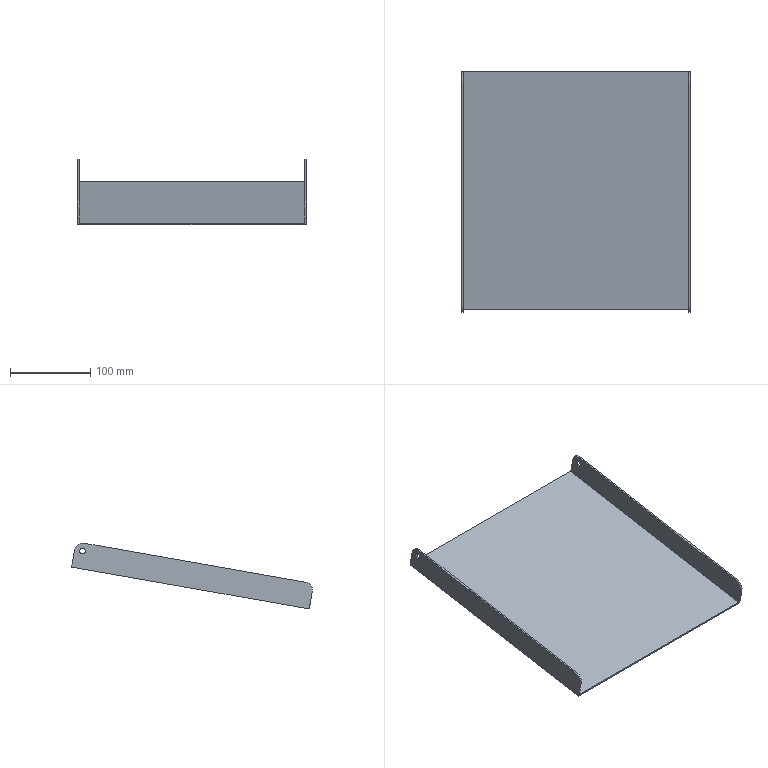Part | NX | features HB 2 | 1 solid | 16 faces | box 285 x 300.028 x 82.132 mm | volume 207104 mm3 | plane 10 | cylinder 6 | commonest cylinder face diameters 20 x4 7 x2
STEP:
#1=CARTESIAN_POINT('',(564.,-684.707,-373.956));
#2=VERTEX_POINT('',#1);
#3=CARTESIAN_POINT('',(564.,-685.612,-377.336));
#4=DIRECTION('',(1.,0.,0.));
#5=DIRECTION('',(0.,0.2588,0.9659));
#6=AXIS2_PLACEMENT_3D('',#3,#4,#5);
#7=CIRCLE('',#6,3.5);
#8=EDGE_CURVE('',#2,#2,#7,.T.);
#9=ORIENTED_EDGE('',*,*,#8,.F.);
#10=EDGE_LOOP('',(#9));
#11=FACE_BOUND('',#10,.T.);
#12=CARTESIAN_POINT('',(566.,-684.707,-373.956));
#13=VERTEX_POINT('',#12);
#14=CARTESIAN_POINT('',(566.,-685.612,-377.336));
#15=DIRECTION('',(-1.,0.,0.));
#16=DIRECTION('',(0.,0.2588,0.9659));
#17=AXIS2_PLACEMENT_3D('',#14,#15,#16);
#18=CIRCLE('',#17,3.5);
#19=EDGE_CURVE('',#13,#13,#18,.T.);
#20=ORIENTED_EDGE('',*,*,#19,.F.);
#21=EDGE_LOOP('',(#20));
#22=FACE_BOUND('',#21,.T.);
#23=CARTESIAN_POINT('',(1166.,-685.612,-377.336));
#24=DIRECTION('',(-1.,0.,0.));
#25=DIRECTION('',(0.,-0.2588,-0.9659));
#26=AXIS2_PLACEMENT_3D('',#23,#24,#25);
#27=CYLINDRICAL_SURFACE('',#26,3.5);
#28=ADVANCED_FACE('',(#11,#22),#27,.F.);
#29=CARTESIAN_POINT('',(564.,-687.349,-367.488));
#30=VERTEX_POINT('',#29);
#31=CARTESIAN_POINT('',(564.,-963.709,-416.218));
#32=VERTEX_POINT('',#31);
#33=CARTESIAN_POINT('',(564.,-562.892,-345.543));
#34=DIRECTION('',(0.,-0.9848,-0.1736));
#35=VECTOR('',#34,1000.);
#36=LINE('',#33,#35);
#37=EDGE_CURVE('',#30,#32,#36,.T.);
#38=ORIENTED_EDGE('',*,*,#37,.T.);
#39=CARTESIAN_POINT('',(566.,-963.709,-416.218));
#40=VERTEX_POINT('',#39);
#41=CARTESIAN_POINT('',(560.,-963.709,-416.218));
#42=DIRECTION('',(1.,0.,0.));
#43=VECTOR('',#42,1000.);
#44=LINE('',#41,#43);
#45=EDGE_CURVE('',#32,#40,#44,.T.);
#46=ORIENTED_EDGE('',*,*,#45,.T.);
#47=CARTESIAN_POINT('',(566.,-687.349,-367.488));
#48=VERTEX_POINT('',#47);
#49=CARTESIAN_POINT('',(566.,-562.892,-345.543));
#50=DIRECTION('',(0.,-0.9848,-0.1736));
#51=VECTOR('',#50,1000.);
#52=LINE('',#49,#51);
#53=EDGE_CURVE('',#48,#40,#52,.T.);
#54=ORIENTED_EDGE('',*,*,#53,.F.);
#55=CARTESIAN_POINT('',(560.,-687.349,-367.488));
#56=DIRECTION('',(1.,0.,0.));
#57=VECTOR('',#56,1000.);
#58=LINE('',#55,#57);
#59=EDGE_CURVE('',#30,#48,#58,.T.);
#60=ORIENTED_EDGE('',*,*,#59,.F.);
#61=EDGE_LOOP('',(#38,#46,#54,#60));
#62=FACE_BOUND('',#61,.T.);
#63=CARTESIAN_POINT('',(560.,-562.892,-345.543));
#64=DIRECTION('',(0.,0.1736,-0.9848));
#65=DIRECTION('',(0.,-0.9848,-0.1736));
#66=AXIS2_PLACEMENT_3D('',#63,#64,#65);
#67=PLANE('',#66);
#68=ADVANCED_FACE('',(#62),#67,.F.);
#69=CARTESIAN_POINT('',(564.,-971.82,-427.803));
#70=VERTEX_POINT('',#69);
#71=CARTESIAN_POINT('',(564.,-961.972,-426.066));
#72=DIRECTION('',(-1.,0.,0.));
#73=DIRECTION('',(0.,0.2588,0.9659));
#74=AXIS2_PLACEMENT_3D('',#71,#72,#73);
#75=CIRCLE('',#74,10.);
#76=EDGE_CURVE('',#70,#32,#75,.T.);
#77=ORIENTED_EDGE('',*,*,#76,.F.);
#78=CARTESIAN_POINT('',(566.,-971.82,-427.803));
#79=VERTEX_POINT('',#78);
#80=CARTESIAN_POINT('',(520.,-971.82,-427.803));
#81=DIRECTION('',(-1.,0.,0.));
#82=VECTOR('',#81,1000.);
#83=LINE('',#80,#82);
#84=EDGE_CURVE('',#79,#70,#83,.T.);
#85=ORIENTED_EDGE('',*,*,#84,.F.);
#86=CARTESIAN_POINT('',(566.,-961.972,-426.066));
#87=DIRECTION('',(1.,0.,0.));
#88=DIRECTION('',(0.,0.2588,0.9659));
#89=AXIS2_PLACEMENT_3D('',#86,#87,#88);
#90=CIRCLE('',#89,10.);
#91=EDGE_CURVE('',#40,#79,#90,.T.);
#92=ORIENTED_EDGE('',*,*,#91,.F.);
#93=ORIENTED_EDGE('',*,*,#45,.F.);
#94=EDGE_LOOP('',(#77,#85,#92,#93));
#95=FACE_BOUND('',#94,.T.);
#96=CARTESIAN_POINT('',(560.,-961.972,-426.066));
#97=DIRECTION('',(1.,0.,0.));
#98=DIRECTION('',(0.,0.2588,0.9659));
#99=AXIS2_PLACEMENT_3D('',#96,#97,#98);
#100=CYLINDRICAL_SURFACE('',#99,10.);
#101=ADVANCED_FACE('',(#95),#100,.T.);
#102=ORIENTED_EDGE('',*,*,#53,.T.);
#103=ORIENTED_EDGE('',*,*,#91,.T.);
#104=CARTESIAN_POINT('',(566.,-968.,-449.468));
#105=VERTEX_POINT('',#104);
#106=CARTESIAN_POINT('',(566.,-968.347,-447.499));
#107=DIRECTION('',(0.,0.1736,-0.9848));
#108=VECTOR('',#107,1000.);
#109=LINE('',#106,#108);
#110=EDGE_CURVE('',#79,#105,#109,.T.);
#111=ORIENTED_EDGE('',*,*,#110,.T.);
#112=CARTESIAN_POINT('',(566.,-671.944,-397.266));
#113=VERTEX_POINT('',#112);
#114=CARTESIAN_POINT('',(566.,-557.335,-377.057));
#115=DIRECTION('',(0.,0.9848,0.1736));
#116=VECTOR('',#115,1000.);
#117=LINE('',#114,#116);
#118=EDGE_CURVE('',#105,#113,#117,.T.);
#119=ORIENTED_EDGE('',*,*,#118,.T.);
#120=CARTESIAN_POINT('',(566.,-675.764,-375.6));
#121=VERTEX_POINT('',#120);
#122=CARTESIAN_POINT('',(566.,-672.291,-395.296));
#123=DIRECTION('',(0.,0.1736,-0.9848));
#124=VECTOR('',#123,1000.);
#125=LINE('',#122,#124);
#126=EDGE_CURVE('',#121,#113,#125,.T.);
#127=ORIENTED_EDGE('',*,*,#126,.F.);
#128=CARTESIAN_POINT('',(566.,-685.612,-377.336));
#129=DIRECTION('',(-1.,0.,0.));
#130=DIRECTION('',(0.,-0.5736,0.8192));
#131=AXIS2_PLACEMENT_3D('',#128,#129,#130);
#132=CIRCLE('',#131,10.);
#133=EDGE_CURVE('',#48,#121,#132,.T.);
#134=ORIENTED_EDGE('',*,*,#133,.F.);
#135=EDGE_LOOP('',(#102,#103,#111,#119,#127,#134));
#136=FACE_BOUND('',#135,.T.);
#137=ORIENTED_EDGE('',*,*,#19,.T.);
#138=EDGE_LOOP('',(#137));
#139=FACE_BOUND('',#138,.T.);
#140=CARTESIAN_POINT('',(566.,-557.683,-375.087));
#141=DIRECTION('',(-1.,0.,0.));
#142=DIRECTION('',(0.,-0.2588,-0.9659));
#143=AXIS2_PLACEMENT_3D('',#140,#141,#142);
#144=PLANE('',#143);
#145=ADVANCED_FACE('',(#136,#139),#144,.F.);
#146=CARTESIAN_POINT('',(564.,-675.764,-375.6));
#147=VERTEX_POINT('',#146);
#148=CARTESIAN_POINT('',(564.,-685.612,-377.336));
#149=DIRECTION('',(1.,0.,0.));
#150=DIRECTION('',(0.,-0.5736,0.8192));
#151=AXIS2_PLACEMENT_3D('',#148,#149,#150);
#152=CIRCLE('',#151,10.);
#153=EDGE_CURVE('',#147,#30,#152,.T.);
#154=ORIENTED_EDGE('',*,*,#153,.T.);
#155=ORIENTED_EDGE('',*,*,#59,.T.);
#156=ORIENTED_EDGE('',*,*,#133,.T.);
#157=CARTESIAN_POINT('',(560.,-675.764,-375.6));
#158=DIRECTION('',(-1.,0.,0.));
#159=VECTOR('',#158,1000.);
#160=LINE('',#157,#159);
#161=EDGE_CURVE('',#121,#147,#160,.T.);
#162=ORIENTED_EDGE('',*,*,#161,.T.);
#163=EDGE_LOOP('',(#154,#155,#156,#162));
#164=FACE_BOUND('',#163,.T.);
#165=CARTESIAN_POINT('',(560.,-685.612,-377.336));
#166=DIRECTION('',(1.,0.,0.));
#167=DIRECTION('',(0.,-0.5736,0.8192));
#168=AXIS2_PLACEMENT_3D('',#165,#166,#167);
#169=CYLINDRICAL_SURFACE('',#168,10.);
#170=ADVANCED_FACE('',(#164),#169,.T.);
#171=ORIENTED_EDGE('',*,*,#76,.T.);
#172=ORIENTED_EDGE('',*,*,#37,.F.);
#173=ORIENTED_EDGE('',*,*,#153,.F.);
#174=CARTESIAN_POINT('',(564.,-672.291,-395.296));
#175=VERTEX_POINT('',#174);
#176=CARTESIAN_POINT('',(564.,-672.291,-395.296));
#177=DIRECTION('',(0.,0.1736,-0.9848));
#178=VECTOR('',#177,1000.);
#179=LINE('',#176,#178);
#180=EDGE_CURVE('',#147,#175,#179,.T.);
#181=ORIENTED_EDGE('',*,*,#180,.T.);
#182=CARTESIAN_POINT('',(564.,-968.347,-447.499));
#183=VERTEX_POINT('',#182);
#184=CARTESIAN_POINT('',(564.,-557.683,-375.087));
#185=DIRECTION('',(0.,-0.9848,-0.1736));
#186=VECTOR('',#185,1000.);
#187=LINE('',#184,#186);
#188=EDGE_CURVE('',#175,#183,#187,.T.);
#189=ORIENTED_EDGE('',*,*,#188,.T.);
#190=CARTESIAN_POINT('',(564.,-968.347,-447.499));
#191=DIRECTION('',(0.,0.1736,-0.9848));
#192=VECTOR('',#191,1000.);
#193=LINE('',#190,#192);
#194=EDGE_CURVE('',#70,#183,#193,.T.);
#195=ORIENTED_EDGE('',*,*,#194,.F.);
#196=EDGE_LOOP('',(#171,#172,#173,#181,#189,#195));
#197=FACE_BOUND('',#196,.T.);
#198=ORIENTED_EDGE('',*,*,#8,.T.);
#199=EDGE_LOOP('',(#198));
#200=FACE_BOUND('',#199,.T.);
#201=CARTESIAN_POINT('',(564.,-557.683,-375.087));
#202=DIRECTION('',(-1.,0.,0.));
#203=DIRECTION('',(0.,0.2588,0.9659));
#204=AXIS2_PLACEMENT_3D('',#201,#202,#203);
#205=PLANE('',#204);
#206=ADVANCED_FACE('',(#197,#200),#205,.T.);
#207=CARTESIAN_POINT('',(283.,-672.291,-395.296));
#208=VERTEX_POINT('',#207);
#209=CARTESIAN_POINT('',(520.,-672.291,-395.296));
#210=DIRECTION('',(1.,0.,0.));
#211=VECTOR('',#210,1000.);
#212=LINE('',#209,#211);
#213=EDGE_CURVE('',#208,#175,#212,.T.);
#214=ORIENTED_EDGE('',*,*,#213,.T.);
#215=ORIENTED_EDGE('',*,*,#180,.F.);
#216=ORIENTED_EDGE('',*,*,#161,.F.);
#217=ORIENTED_EDGE('',*,*,#126,.T.);
#218=CARTESIAN_POINT('',(281.,-671.944,-397.266));
#219=VERTEX_POINT('',#218);
#220=CARTESIAN_POINT('',(520.,-671.944,-397.266));
#221=DIRECTION('',(1.,0.,0.));
#222=VECTOR('',#221,1000.);
#223=LINE('',#220,#222);
#224=EDGE_CURVE('',#219,#113,#223,.T.);
#225=ORIENTED_EDGE('',*,*,#224,.F.);
#226=CARTESIAN_POINT('',(281.,-675.764,-375.6));
#227=VERTEX_POINT('',#226);
#228=CARTESIAN_POINT('',(281.,-672.291,-395.296));
#229=DIRECTION('',(0.,0.1736,-0.9848));
#230=VECTOR('',#229,1000.);
#231=LINE('',#228,#230);
#232=EDGE_CURVE('',#227,#219,#231,.T.);
#233=ORIENTED_EDGE('',*,*,#232,.F.);
#234=CARTESIAN_POINT('',(283.,-675.764,-375.6));
#235=VERTEX_POINT('',#234);
#236=CARTESIAN_POINT('',(586.,-675.764,-375.6));
#237=DIRECTION('',(-1.,0.,0.));
#238=VECTOR('',#237,1000.);
#239=LINE('',#236,#238);
#240=EDGE_CURVE('',#235,#227,#239,.T.);
#241=ORIENTED_EDGE('',*,*,#240,.F.);
#242=CARTESIAN_POINT('',(283.,-672.291,-395.296));
#243=DIRECTION('',(0.,0.1736,-0.9848));
#244=VECTOR('',#243,1000.);
#245=LINE('',#242,#244);
#246=EDGE_CURVE('',#235,#208,#245,.T.);
#247=ORIENTED_EDGE('',*,*,#246,.T.);
#248=EDGE_LOOP('',(#214,#215,#216,#217,#225,#233,#241,#247));
#249=FACE_BOUND('',#248,.T.);
#250=CARTESIAN_POINT('',(520.,-672.291,-395.296));
#251=DIRECTION('',(0.,-0.9848,-0.1736));
#252=DIRECTION('',(0.,0.1736,-0.9848));
#253=AXIS2_PLACEMENT_3D('',#250,#251,#252);
#254=PLANE('',#253);
#255=ADVANCED_FACE('',(#249),#254,.F.);
#256=ORIENTED_EDGE('',*,*,#194,.T.);
#257=CARTESIAN_POINT('',(283.,-968.347,-447.499));
#258=VERTEX_POINT('',#257);
#259=CARTESIAN_POINT('',(520.,-968.347,-447.499));
#260=DIRECTION('',(1.,0.,0.));
#261=VECTOR('',#260,1000.);
#262=LINE('',#259,#261);
#263=EDGE_CURVE('',#258,#183,#262,.T.);
#264=ORIENTED_EDGE('',*,*,#263,.F.);
#265=CARTESIAN_POINT('',(283.,-971.82,-427.803));
#266=VERTEX_POINT('',#265);
#267=CARTESIAN_POINT('',(283.,-968.347,-447.499));
#268=DIRECTION('',(0.,0.1736,-0.9848));
#269=VECTOR('',#268,1000.);
#270=LINE('',#267,#269);
#271=EDGE_CURVE('',#266,#258,#270,.T.);
#272=ORIENTED_EDGE('',*,*,#271,.F.);
#273=CARTESIAN_POINT('',(281.,-971.82,-427.803));
#274=VERTEX_POINT('',#273);
#275=CARTESIAN_POINT('',(520.,-971.82,-427.803));
#276=DIRECTION('',(-1.,0.,0.));
#277=VECTOR('',#276,1000.);
#278=LINE('',#275,#277);
#279=EDGE_CURVE('',#266,#274,#278,.T.);
#280=ORIENTED_EDGE('',*,*,#279,.T.);
#281=CARTESIAN_POINT('',(281.,-968.,-449.468));
#282=VERTEX_POINT('',#281);
#283=CARTESIAN_POINT('',(281.,-968.347,-447.499));
#284=DIRECTION('',(0.,0.1736,-0.9848));
#285=VECTOR('',#284,1000.);
#286=LINE('',#283,#285);
#287=EDGE_CURVE('',#274,#282,#286,.T.);
#288=ORIENTED_EDGE('',*,*,#287,.T.);
#289=CARTESIAN_POINT('',(520.,-968.,-449.468));
#290=DIRECTION('',(1.,0.,0.));
#291=VECTOR('',#290,1000.);
#292=LINE('',#289,#291);
#293=EDGE_CURVE('',#282,#105,#292,.T.);
#294=ORIENTED_EDGE('',*,*,#293,.T.);
#295=ORIENTED_EDGE('',*,*,#110,.F.);
#296=ORIENTED_EDGE('',*,*,#84,.T.);
#297=EDGE_LOOP('',(#256,#264,#272,#280,#288,#294,#295,#296));
#298=FACE_BOUND('',#297,.T.);
#299=CARTESIAN_POINT('',(520.,-968.347,-447.499));
#300=DIRECTION('',(0.,0.9848,0.1736));
#301=DIRECTION('',(0.,0.1736,-0.9848));
#302=AXIS2_PLACEMENT_3D('',#299,#300,#301);
#303=PLANE('',#302);
#304=ADVANCED_FACE('',(#298),#303,.F.);
#305=ORIENTED_EDGE('',*,*,#118,.F.);
#306=ORIENTED_EDGE('',*,*,#293,.F.);
#307=CARTESIAN_POINT('',(281.,-557.335,-377.057));
#308=DIRECTION('',(0.,-0.9848,-0.1736));
#309=VECTOR('',#308,1000.);
#310=LINE('',#307,#309);
#311=EDGE_CURVE('',#219,#282,#310,.T.);
#312=ORIENTED_EDGE('',*,*,#311,.F.);
#313=ORIENTED_EDGE('',*,*,#224,.T.);
#314=EDGE_LOOP('',(#305,#306,#312,#313));
#315=FACE_BOUND('',#314,.T.);
#316=CARTESIAN_POINT('',(520.,-557.335,-377.057));
#317=DIRECTION('',(0.,-0.1736,0.9848));
#318=DIRECTION('',(-1.,0.,0.));
#319=AXIS2_PLACEMENT_3D('',#316,#317,#318);
#320=PLANE('',#319);
#321=ADVANCED_FACE('',(#315),#320,.F.);
#322=ORIENTED_EDGE('',*,*,#263,.T.);
#323=ORIENTED_EDGE('',*,*,#188,.F.);
#324=ORIENTED_EDGE('',*,*,#213,.F.);
#325=CARTESIAN_POINT('',(283.,-557.683,-375.087));
#326=DIRECTION('',(0.,0.9848,0.1736));
#327=VECTOR('',#326,1000.);
#328=LINE('',#325,#327);
#329=EDGE_CURVE('',#258,#208,#328,.T.);
#330=ORIENTED_EDGE('',*,*,#329,.F.);
#331=EDGE_LOOP('',(#322,#323,#324,#330));
#332=FACE_BOUND('',#331,.T.);
#333=CARTESIAN_POINT('',(520.,-557.683,-375.087));
#334=DIRECTION('',(0.,-0.1736,0.9848));
#335=DIRECTION('',(-1.,0.,0.));
#336=AXIS2_PLACEMENT_3D('',#333,#334,#335);
#337=PLANE('',#336);
#338=ADVANCED_FACE('',(#332),#337,.T.);
#339=CARTESIAN_POINT('',(281.,-686.518,-380.717));
#340=VERTEX_POINT('',#339);
#341=CARTESIAN_POINT('',(281.,-685.612,-377.336));
#342=DIRECTION('',(1.,0.,0.));
#343=DIRECTION('',(0.,-0.2588,-0.9659));
#344=AXIS2_PLACEMENT_3D('',#341,#342,#343);
#345=CIRCLE('',#344,3.5);
#346=EDGE_CURVE('',#340,#340,#345,.T.);
#347=ORIENTED_EDGE('',*,*,#346,.T.);
#348=EDGE_LOOP('',(#347));
#349=FACE_BOUND('',#348,.T.);
#350=ORIENTED_EDGE('',*,*,#311,.T.);
#351=ORIENTED_EDGE('',*,*,#287,.F.);
#352=CARTESIAN_POINT('',(281.,-963.709,-416.218));
#353=VERTEX_POINT('',#352);
#354=CARTESIAN_POINT('',(281.,-961.972,-426.066));
#355=DIRECTION('',(-1.,0.,0.));
#356=DIRECTION('',(0.,-0.2588,-0.9659));
#357=AXIS2_PLACEMENT_3D('',#354,#355,#356);
#358=CIRCLE('',#357,10.);
#359=EDGE_CURVE('',#274,#353,#358,.T.);
#360=ORIENTED_EDGE('',*,*,#359,.T.);
#361=CARTESIAN_POINT('',(281.,-687.349,-367.488));
#362=VERTEX_POINT('',#361);
#363=CARTESIAN_POINT('',(281.,-562.892,-345.543));
#364=DIRECTION('',(0.,-0.9848,-0.1736));
#365=VECTOR('',#364,1000.);
#366=LINE('',#363,#365);
#367=EDGE_CURVE('',#362,#353,#366,.T.);
#368=ORIENTED_EDGE('',*,*,#367,.F.);
#369=CARTESIAN_POINT('',(281.,-685.612,-377.336));
#370=DIRECTION('',(1.,0.,0.));
#371=DIRECTION('',(0.,0.5736,-0.8192));
#372=AXIS2_PLACEMENT_3D('',#369,#370,#371);
#373=CIRCLE('',#372,10.);
#374=EDGE_CURVE('',#227,#362,#373,.T.);
#375=ORIENTED_EDGE('',*,*,#374,.F.);
#376=ORIENTED_EDGE('',*,*,#232,.T.);
#377=EDGE_LOOP('',(#350,#351,#360,#368,#375,#376));
#378=FACE_BOUND('',#377,.T.);
#379=CARTESIAN_POINT('',(281.,-557.683,-375.087));
#380=DIRECTION('',(1.,0.,0.));
#381=DIRECTION('',(0.,0.2588,0.9659));
#382=AXIS2_PLACEMENT_3D('',#379,#380,#381);
#383=PLANE('',#382);
#384=ADVANCED_FACE('',(#349,#378),#383,.F.);
#385=ORIENTED_EDGE('',*,*,#367,.T.);
#386=CARTESIAN_POINT('',(283.,-963.709,-416.218));
#387=VERTEX_POINT('',#386);
#388=CARTESIAN_POINT('',(328.,-963.709,-416.218));
#389=DIRECTION('',(1.,0.,0.));
#390=VECTOR('',#389,1000.);
#391=LINE('',#388,#390);
#392=EDGE_CURVE('',#353,#387,#391,.T.);
#393=ORIENTED_EDGE('',*,*,#392,.T.);
#394=CARTESIAN_POINT('',(283.,-687.349,-367.488));
#395=VERTEX_POINT('',#394);
#396=CARTESIAN_POINT('',(283.,-562.892,-345.543));
#397=DIRECTION('',(0.,-0.9848,-0.1736));
#398=VECTOR('',#397,1000.);
#399=LINE('',#396,#398);
#400=EDGE_CURVE('',#395,#387,#399,.T.);
#401=ORIENTED_EDGE('',*,*,#400,.F.);
#402=CARTESIAN_POINT('',(328.,-687.349,-367.488));
#403=DIRECTION('',(1.,0.,0.));
#404=VECTOR('',#403,1000.);
#405=LINE('',#402,#404);
#406=EDGE_CURVE('',#362,#395,#405,.T.);
#407=ORIENTED_EDGE('',*,*,#406,.F.);
#408=EDGE_LOOP('',(#385,#393,#401,#407));
#409=FACE_BOUND('',#408,.T.);
#410=CARTESIAN_POINT('',(328.,-562.892,-345.543));
#411=DIRECTION('',(0.,0.1736,-0.9848));
#412=DIRECTION('',(0.,-0.9848,-0.1736));
#413=AXIS2_PLACEMENT_3D('',#410,#411,#412);
#414=PLANE('',#413);
#415=ADVANCED_FACE('',(#409),#414,.F.);
#416=CARTESIAN_POINT('',(283.,-686.518,-380.717));
#417=VERTEX_POINT('',#416);
#418=CARTESIAN_POINT('',(283.,-685.612,-377.336));
#419=DIRECTION('',(1.,0.,0.));
#420=DIRECTION('',(0.,-0.2588,-0.9659));
#421=AXIS2_PLACEMENT_3D('',#418,#419,#420);
#422=CIRCLE('',#421,3.5);
#423=EDGE_CURVE('',#417,#417,#422,.T.);
#424=ORIENTED_EDGE('',*,*,#423,.F.);
#425=EDGE_LOOP('',(#424));
#426=FACE_BOUND('',#425,.T.);
#427=ORIENTED_EDGE('',*,*,#329,.T.);
#428=ORIENTED_EDGE('',*,*,#246,.F.);
#429=CARTESIAN_POINT('',(283.,-685.612,-377.336));
#430=DIRECTION('',(-1.,0.,0.));
#431=DIRECTION('',(0.,0.5736,-0.8192));
#432=AXIS2_PLACEMENT_3D('',#429,#430,#431);
#433=CIRCLE('',#432,10.);
#434=EDGE_CURVE('',#395,#235,#433,.T.);
#435=ORIENTED_EDGE('',*,*,#434,.F.);
#436=ORIENTED_EDGE('',*,*,#400,.T.);
#437=CARTESIAN_POINT('',(283.,-961.972,-426.066));
#438=DIRECTION('',(1.,0.,0.));
#439=DIRECTION('',(0.,-0.2588,-0.9659));
#440=AXIS2_PLACEMENT_3D('',#437,#438,#439);
#441=CIRCLE('',#440,10.);
#442=EDGE_CURVE('',#387,#266,#441,.T.);
#443=ORIENTED_EDGE('',*,*,#442,.T.);
#444=ORIENTED_EDGE('',*,*,#271,.T.);
#445=EDGE_LOOP('',(#427,#428,#435,#436,#443,#444));
#446=FACE_BOUND('',#445,.T.);
#447=CARTESIAN_POINT('',(283.,-557.683,-375.087));
#448=DIRECTION('',(1.,0.,0.));
#449=DIRECTION('',(0.,0.2588,0.9659));
#450=AXIS2_PLACEMENT_3D('',#447,#448,#449);
#451=PLANE('',#450);
#452=ADVANCED_FACE('',(#426,#446),#451,.T.);
#453=ORIENTED_EDGE('',*,*,#442,.F.);
#454=ORIENTED_EDGE('',*,*,#392,.F.);
#455=ORIENTED_EDGE('',*,*,#359,.F.);
#456=ORIENTED_EDGE('',*,*,#279,.F.);
#457=EDGE_LOOP('',(#453,#454,#455,#456));
#458=FACE_BOUND('',#457,.T.);
#459=CARTESIAN_POINT('',(586.,-961.972,-426.066));
#460=DIRECTION('',(-1.,0.,0.));
#461=DIRECTION('',(0.,-0.2588,-0.9659));
#462=AXIS2_PLACEMENT_3D('',#459,#460,#461);
#463=CYLINDRICAL_SURFACE('',#462,10.);
#464=ADVANCED_FACE('',(#458),#463,.T.);
#465=ORIENTED_EDGE('',*,*,#434,.T.);
#466=ORIENTED_EDGE('',*,*,#240,.T.);
#467=ORIENTED_EDGE('',*,*,#374,.T.);
#468=ORIENTED_EDGE('',*,*,#406,.T.);
#469=EDGE_LOOP('',(#465,#466,#467,#468));
#470=FACE_BOUND('',#469,.T.);
#471=CARTESIAN_POINT('',(586.,-685.612,-377.336));
#472=DIRECTION('',(-1.,0.,0.));
#473=DIRECTION('',(0.,0.5736,-0.8192));
#474=AXIS2_PLACEMENT_3D('',#471,#472,#473);
#475=CYLINDRICAL_SURFACE('',#474,10.);
#476=ADVANCED_FACE('',(#470),#475,.T.);
#477=ORIENTED_EDGE('',*,*,#423,.T.);
#478=EDGE_LOOP('',(#477));
#479=FACE_BOUND('',#478,.T.);
#480=ORIENTED_EDGE('',*,*,#346,.F.);
#481=EDGE_LOOP('',(#480));
#482=FACE_BOUND('',#481,.T.);
#483=CARTESIAN_POINT('',(326.,-685.612,-377.336));
#484=DIRECTION('',(1.,0.,0.));
#485=DIRECTION('',(0.,0.2588,0.9659));
#486=AXIS2_PLACEMENT_3D('',#483,#484,#485);
#487=CYLINDRICAL_SURFACE('',#486,3.5);
#488=ADVANCED_FACE('',(#479,#482),#487,.F.);
#489=CLOSED_SHELL('',(#28,#68,#101,#145,#170,#206,#255,#304,#321,#338,#384,#415,#452,#464,#476,#488));
#490=MANIFOLD_SOLID_BREP('',#489);
#491=(LENGTH_UNIT()NAMED_UNIT(*)SI_UNIT(.MILLI.,.METRE.));
#492=UNCERTAINTY_MEASURE_WITH_UNIT(LENGTH_MEASURE(0.00001),#491,'','');
#493=(NAMED_UNIT(*)PLANE_ANGLE_UNIT()SI_UNIT($,.RADIAN.));
#494=(NAMED_UNIT(*)SI_UNIT($,.STERADIAN.)SOLID_ANGLE_UNIT());
#495=(GEOMETRIC_REPRESENTATION_CONTEXT(3)GLOBAL_UNCERTAINTY_ASSIGNED_CONTEXT((#492))GLOBAL_UNIT_ASSIGNED_CONTEXT((#491,#493,#494))REPRESENTATION_CONTEXT('',''));
#496=ADVANCED_BREP_SHAPE_REPRESENTATION('',(#490),#495);